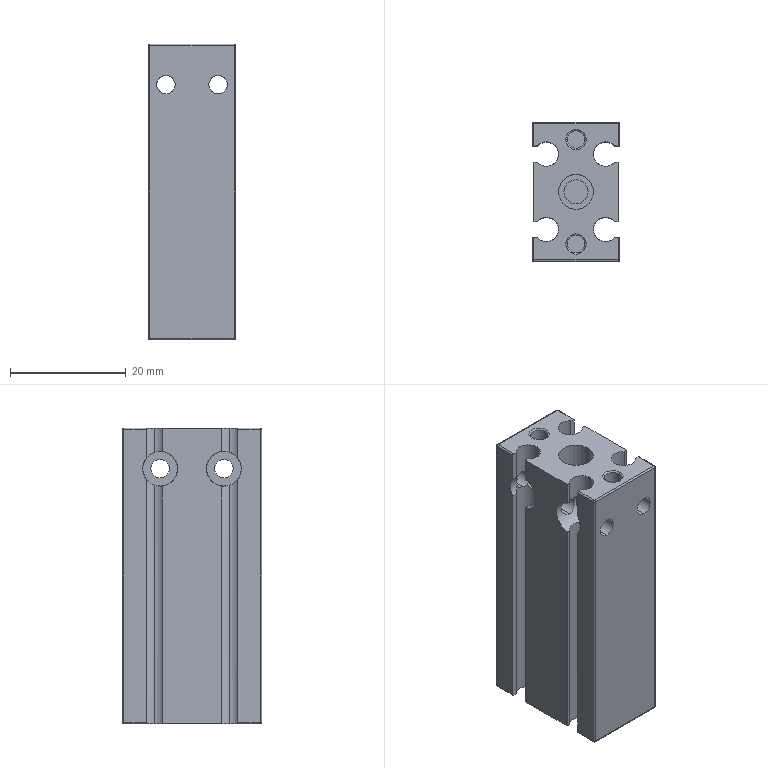Part | NX | 1 solid | 141 faces | box 15 x 24 x 51 mm | volume 11990 mm3 | cylinder 80 | plane 41 | torus 8 | sphere 8 | cone 4 | commonest cylinder face diameters 0.5 x16 3.2 x16 6 x14 4.2 x12 3 x8 0.8 x4